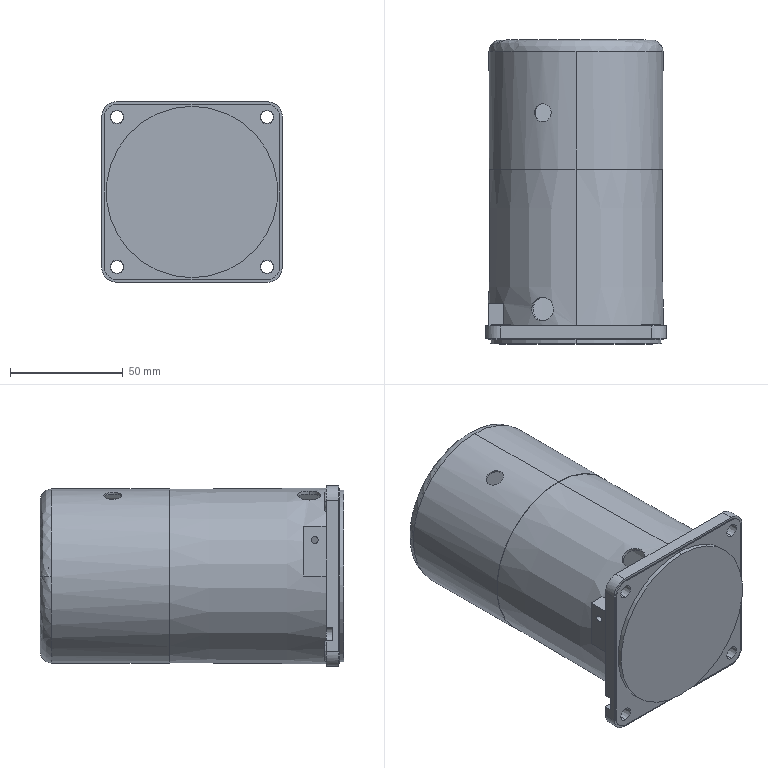Part | SolidWorks | 1 solid | 93 faces | box 79.972 x 134.7 x 79.972 mm | volume 165976 mm3 | plane 33 | cylinder 28 | spline 18 | cone 14 | commonest cylinder face diameters 4.5 x4 12 x4 13 x4 3 x2 6 x2 8 x2